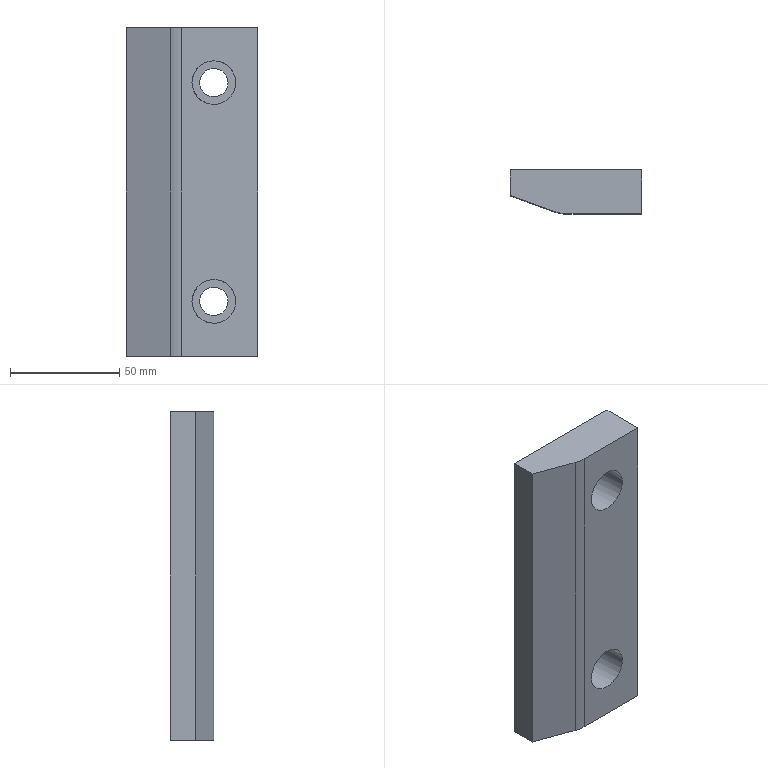Part | NX | features MAIN_BODY 2 | 1 solid | 14 faces | box 60 x 20 x 150 mm | volume 155051 mm3 | plane 9 | cylinder 5 | commonest cylinder face diameters 13 x2 20 x2 30 x1
STEP:
#1=CARTESIAN_POINT('',(-46.,-365.,-205.));
#2=VERTEX_POINT('',#1);
#3=CARTESIAN_POINT('',(14.,-365.,-205.));
#4=VERTEX_POINT('',#3);
#5=CARTESIAN_POINT('',(-71.,-365.,-205.));
#6=DIRECTION('',(1.,0.,0.));
#7=VECTOR('',#6,1000.);
#8=LINE('',#5,#7);
#9=EDGE_CURVE('',#2,#4,#8,.T.);
#10=ORIENTED_EDGE('',*,*,#9,.F.);
#11=CARTESIAN_POINT('',(-46.,-365.,-55.));
#12=VERTEX_POINT('',#11);
#13=CARTESIAN_POINT('',(-46.,-365.,-130.));
#14=DIRECTION('',(0.,0.,-1.));
#15=VECTOR('',#14,1000.);
#16=LINE('',#13,#15);
#17=EDGE_CURVE('',#12,#2,#16,.T.);
#18=ORIENTED_EDGE('',*,*,#17,.F.);
#19=CARTESIAN_POINT('',(14.,-365.,-55.));
#20=VERTEX_POINT('',#19);
#21=CARTESIAN_POINT('',(-71.,-365.,-55.));
#22=DIRECTION('',(-1.,0.,0.));
#23=VECTOR('',#22,1000.);
#24=LINE('',#21,#23);
#25=EDGE_CURVE('',#20,#12,#24,.T.);
#26=ORIENTED_EDGE('',*,*,#25,.F.);
#27=CARTESIAN_POINT('',(14.,-365.,-130.));
#28=DIRECTION('',(0.,0.,1.));
#29=VECTOR('',#28,1000.);
#30=LINE('',#27,#29);
#31=EDGE_CURVE('',#4,#20,#30,.T.);
#32=ORIENTED_EDGE('',*,*,#31,.F.);
#33=EDGE_LOOP('',(#10,#18,#26,#32));
#34=FACE_BOUND('',#33,.T.);
#35=CARTESIAN_POINT('',(-12.5,-365.,-180.));
#36=VERTEX_POINT('',#35);
#37=CARTESIAN_POINT('',(-6.,-365.,-180.));
#38=DIRECTION('',(0.,1.,0.));
#39=DIRECTION('',(-1.,0.,0.));
#40=AXIS2_PLACEMENT_3D('',#37,#38,#39);
#41=CIRCLE('',#40,6.5);
#42=EDGE_CURVE('',#36,#36,#41,.T.);
#43=ORIENTED_EDGE('',*,*,#42,.F.);
#44=EDGE_LOOP('',(#43));
#45=FACE_BOUND('',#44,.T.);
#46=CARTESIAN_POINT('',(-12.5,-365.,-80.));
#47=VERTEX_POINT('',#46);
#48=CARTESIAN_POINT('',(-6.,-365.,-80.));
#49=DIRECTION('',(0.,1.,0.));
#50=DIRECTION('',(-1.,0.,0.));
#51=AXIS2_PLACEMENT_3D('',#48,#49,#50);
#52=CIRCLE('',#51,6.5);
#53=EDGE_CURVE('',#47,#47,#52,.T.);
#54=ORIENTED_EDGE('',*,*,#53,.F.);
#55=EDGE_LOOP('',(#54));
#56=FACE_BOUND('',#55,.T.);
#57=CARTESIAN_POINT('',(-71.,-365.,-130.));
#58=DIRECTION('',(0.,1.,0.));
#59=DIRECTION('',(-1.,0.,0.));
#60=AXIS2_PLACEMENT_3D('',#57,#58,#59);
#61=PLANE('',#60);
#62=ADVANCED_FACE('',(#34,#45,#56),#61,.T.);
#63=CARTESIAN_POINT('',(14.,-385.,-205.));
#64=VERTEX_POINT('',#63);
#65=CARTESIAN_POINT('',(-20.598,-385.,-205.));
#66=VERTEX_POINT('',#65);
#67=CARTESIAN_POINT('',(-71.,-385.,-205.));
#68=DIRECTION('',(-1.,0.,0.));
#69=VECTOR('',#68,1000.);
#70=LINE('',#67,#69);
#71=EDGE_CURVE('',#64,#66,#70,.T.);
#72=ORIENTED_EDGE('',*,*,#71,.F.);
#73=CARTESIAN_POINT('',(14.,-385.,-55.));
#74=VERTEX_POINT('',#73);
#75=CARTESIAN_POINT('',(14.,-385.,-130.));
#76=DIRECTION('',(0.,0.,-1.));
#77=VECTOR('',#76,1000.);
#78=LINE('',#75,#77);
#79=EDGE_CURVE('',#74,#64,#78,.T.);
#80=ORIENTED_EDGE('',*,*,#79,.F.);
#81=CARTESIAN_POINT('',(-20.598,-385.,-55.));
#82=VERTEX_POINT('',#81);
#83=CARTESIAN_POINT('',(79.,-385.,-55.));
#84=DIRECTION('',(1.,0.,0.));
#85=VECTOR('',#84,1000.);
#86=LINE('',#83,#85);
#87=EDGE_CURVE('',#82,#74,#86,.T.);
#88=ORIENTED_EDGE('',*,*,#87,.F.);
#89=CARTESIAN_POINT('',(-20.598,-385.,-130.));
#90=DIRECTION('',(0.,0.,1.));
#91=VECTOR('',#90,1000.);
#92=LINE('',#89,#91);
#93=EDGE_CURVE('',#66,#82,#92,.T.);
#94=ORIENTED_EDGE('',*,*,#93,.F.);
#95=EDGE_LOOP('',(#72,#80,#88,#94));
#96=FACE_BOUND('',#95,.T.);
#97=CARTESIAN_POINT('',(-6.,-385.,-170.));
#98=VERTEX_POINT('',#97);
#99=CARTESIAN_POINT('',(-6.,-385.,-180.));
#100=DIRECTION('',(0.,-1.,0.));
#101=DIRECTION('',(0.,0.,1.));
#102=AXIS2_PLACEMENT_3D('',#99,#100,#101);
#103=CIRCLE('',#102,10.);
#104=EDGE_CURVE('',#98,#98,#103,.T.);
#105=ORIENTED_EDGE('',*,*,#104,.F.);
#106=EDGE_LOOP('',(#105));
#107=FACE_BOUND('',#106,.T.);
#108=CARTESIAN_POINT('',(-6.,-385.,-70.));
#109=VERTEX_POINT('',#108);
#110=CARTESIAN_POINT('',(-6.,-385.,-80.));
#111=DIRECTION('',(0.,-1.,0.));
#112=DIRECTION('',(0.,0.,1.));
#113=AXIS2_PLACEMENT_3D('',#110,#111,#112);
#114=CIRCLE('',#113,10.);
#115=EDGE_CURVE('',#109,#109,#114,.T.);
#116=ORIENTED_EDGE('',*,*,#115,.F.);
#117=EDGE_LOOP('',(#116));
#118=FACE_BOUND('',#117,.T.);
#119=CARTESIAN_POINT('',(79.,-385.,-130.));
#120=DIRECTION('',(0.,-1.,0.));
#121=DIRECTION('',(0.,0.,1.));
#122=AXIS2_PLACEMENT_3D('',#119,#120,#121);
#123=PLANE('',#122);
#124=ADVANCED_FACE('',(#96,#107,#118),#123,.T.);
#125=CARTESIAN_POINT('',(-46.,-376.717,-55.));
#126=VERTEX_POINT('',#125);
#127=CARTESIAN_POINT('',(-25.729,-384.095,-55.));
#128=VERTEX_POINT('',#127);
#129=CARTESIAN_POINT('',(-8.79,-390.261,-55.));
#130=DIRECTION('',(0.9397,-0.342,0.));
#131=VECTOR('',#130,1000.);
#132=LINE('',#129,#131);
#133=EDGE_CURVE('',#126,#128,#132,.T.);
#134=ORIENTED_EDGE('',*,*,#133,.F.);
#135=CARTESIAN_POINT('',(-46.,-376.717,-205.));
#136=VERTEX_POINT('',#135);
#137=CARTESIAN_POINT('',(-46.,-376.717,-130.));
#138=DIRECTION('',(0.,0.,1.));
#139=VECTOR('',#138,1000.);
#140=LINE('',#137,#139);
#141=EDGE_CURVE('',#136,#126,#140,.T.);
#142=ORIENTED_EDGE('',*,*,#141,.F.);
#143=CARTESIAN_POINT('',(-25.729,-384.095,-205.));
#144=VERTEX_POINT('',#143);
#145=CARTESIAN_POINT('',(-57.618,-372.489,-205.));
#146=DIRECTION('',(-0.9397,0.342,0.));
#147=VECTOR('',#146,1000.);
#148=LINE('',#145,#147);
#149=EDGE_CURVE('',#144,#136,#148,.T.);
#150=ORIENTED_EDGE('',*,*,#149,.F.);
#151=CARTESIAN_POINT('',(-25.729,-384.095,-130.));
#152=DIRECTION('',(0.,0.,1.));
#153=VECTOR('',#152,1000.);
#154=LINE('',#151,#153);
#155=EDGE_CURVE('',#128,#144,#154,.F.);
#156=ORIENTED_EDGE('',*,*,#155,.F.);
#157=EDGE_LOOP('',(#134,#142,#150,#156));
#158=FACE_BOUND('',#157,.T.);
#159=CARTESIAN_POINT('',(-8.79,-390.261,-130.));
#160=DIRECTION('',(-0.342,-0.9397,0.));
#161=DIRECTION('',(0.9397,-0.342,0.));
#162=AXIS2_PLACEMENT_3D('',#159,#160,#161);
#163=PLANE('',#162);
#164=ADVANCED_FACE('',(#158),#163,.T.);
#165=ORIENTED_EDGE('',*,*,#141,.T.);
#166=CARTESIAN_POINT('',(-46.,-395.,-55.));
#167=DIRECTION('',(0.,-1.,0.));
#168=VECTOR('',#167,1000.);
#169=LINE('',#166,#168);
#170=EDGE_CURVE('',#12,#126,#169,.T.);
#171=ORIENTED_EDGE('',*,*,#170,.F.);
#172=ORIENTED_EDGE('',*,*,#17,.T.);
#173=CARTESIAN_POINT('',(-46.,-360.359,-205.));
#174=DIRECTION('',(0.,1.,0.));
#175=VECTOR('',#174,1000.);
#176=LINE('',#173,#175);
#177=EDGE_CURVE('',#136,#2,#176,.T.);
#178=ORIENTED_EDGE('',*,*,#177,.F.);
#179=EDGE_LOOP('',(#165,#171,#172,#178));
#180=FACE_BOUND('',#179,.T.);
#181=CARTESIAN_POINT('',(-46.,-360.359,-130.));
#182=DIRECTION('',(-1.,0.,0.));
#183=DIRECTION('',(0.,0.,-1.));
#184=AXIS2_PLACEMENT_3D('',#181,#182,#183);
#185=PLANE('',#184);
#186=ADVANCED_FACE('',(#180),#185,.T.);
#187=CARTESIAN_POINT('',(14.,-395.,-205.));
#188=DIRECTION('',(0.,-1.,0.));
#189=VECTOR('',#188,1000.);
#190=LINE('',#187,#189);
#191=EDGE_CURVE('',#4,#64,#190,.T.);
#192=ORIENTED_EDGE('',*,*,#191,.F.);
#193=ORIENTED_EDGE('',*,*,#31,.T.);
#194=CARTESIAN_POINT('',(14.,-395.,-55.));
#195=DIRECTION('',(0.,-1.,0.));
#196=VECTOR('',#195,1000.);
#197=LINE('',#194,#196);
#198=EDGE_CURVE('',#20,#74,#197,.T.);
#199=ORIENTED_EDGE('',*,*,#198,.T.);
#200=ORIENTED_EDGE('',*,*,#79,.T.);
#201=EDGE_LOOP('',(#192,#193,#199,#200));
#202=FACE_BOUND('',#201,.T.);
#203=CARTESIAN_POINT('',(14.,-350.,-130.));
#204=DIRECTION('',(1.,0.,0.));
#205=DIRECTION('',(0.,0.,1.));
#206=AXIS2_PLACEMENT_3D('',#203,#204,#205);
#207=PLANE('',#206);
#208=ADVANCED_FACE('',(#202),#207,.T.);
#209=ORIENTED_EDGE('',*,*,#149,.T.);
#210=ORIENTED_EDGE('',*,*,#177,.T.);
#211=ORIENTED_EDGE('',*,*,#9,.T.);
#212=ORIENTED_EDGE('',*,*,#191,.T.);
#213=ORIENTED_EDGE('',*,*,#71,.T.);
#214=CARTESIAN_POINT('',(-20.598,-370.,-205.));
#215=DIRECTION('',(0.,0.,1.));
#216=DIRECTION('',(1.,0.,0.));
#217=AXIS2_PLACEMENT_3D('',#214,#215,#216);
#218=CIRCLE('',#217,15.);
#219=EDGE_CURVE('',#144,#66,#218,.T.);
#220=ORIENTED_EDGE('',*,*,#219,.F.);
#221=EDGE_LOOP('',(#209,#210,#211,#212,#213,#220));
#222=FACE_BOUND('',#221,.T.);
#223=CARTESIAN_POINT('',(-71.,-395.,-205.));
#224=DIRECTION('',(0.,0.,-1.));
#225=DIRECTION('',(1.,0.,0.));
#226=AXIS2_PLACEMENT_3D('',#223,#224,#225);
#227=PLANE('',#226);
#228=ADVANCED_FACE('',(#222),#227,.T.);
#229=ORIENTED_EDGE('',*,*,#42,.T.);
#230=EDGE_LOOP('',(#229));
#231=FACE_BOUND('',#230,.T.);
#232=CARTESIAN_POINT('',(-12.5,-370.,-180.));
#233=VERTEX_POINT('',#232);
#234=CARTESIAN_POINT('',(-6.,-370.,-180.));
#235=DIRECTION('',(0.,1.,0.));
#236=DIRECTION('',(-1.,0.,0.));
#237=AXIS2_PLACEMENT_3D('',#234,#235,#236);
#238=CIRCLE('',#237,6.5);
#239=EDGE_CURVE('',#233,#233,#238,.T.);
#240=ORIENTED_EDGE('',*,*,#239,.F.);
#241=EDGE_LOOP('',(#240));
#242=FACE_BOUND('',#241,.T.);
#243=CARTESIAN_POINT('',(-6.,-350.,-180.));
#244=DIRECTION('',(0.,1.,0.));
#245=DIRECTION('',(0.,0.,-1.));
#246=AXIS2_PLACEMENT_3D('',#243,#244,#245);
#247=CYLINDRICAL_SURFACE('',#246,6.5);
#248=ADVANCED_FACE('',(#231,#242),#247,.F.);
#249=ORIENTED_EDGE('',*,*,#239,.T.);
#250=EDGE_LOOP('',(#249));
#251=FACE_BOUND('',#250,.T.);
#252=CARTESIAN_POINT('',(-16.,-370.,-180.));
#253=VERTEX_POINT('',#252);
#254=CARTESIAN_POINT('',(-6.,-370.,-180.));
#255=DIRECTION('',(0.,1.,0.));
#256=DIRECTION('',(-1.,0.,0.));
#257=AXIS2_PLACEMENT_3D('',#254,#255,#256);
#258=CIRCLE('',#257,10.);
#259=EDGE_CURVE('',#253,#253,#258,.T.);
#260=ORIENTED_EDGE('',*,*,#259,.F.);
#261=EDGE_LOOP('',(#260));
#262=FACE_BOUND('',#261,.T.);
#263=CARTESIAN_POINT('',(19.,-370.,-210.));
#264=DIRECTION('',(0.,1.,0.));
#265=DIRECTION('',(0.,0.,-1.));
#266=AXIS2_PLACEMENT_3D('',#263,#264,#265);
#267=PLANE('',#266);
#268=ADVANCED_FACE('',(#251,#262),#267,.F.);
#269=ORIENTED_EDGE('',*,*,#104,.T.);
#270=EDGE_LOOP('',(#269));
#271=FACE_BOUND('',#270,.T.);
#272=ORIENTED_EDGE('',*,*,#259,.T.);
#273=EDGE_LOOP('',(#272));
#274=FACE_BOUND('',#273,.T.);
#275=CARTESIAN_POINT('',(-6.,-395.,-180.));
#276=DIRECTION('',(0.,1.,0.));
#277=DIRECTION('',(0.,0.,-1.));
#278=AXIS2_PLACEMENT_3D('',#275,#276,#277);
#279=CYLINDRICAL_SURFACE('',#278,10.);
#280=ADVANCED_FACE('',(#271,#274),#279,.F.);
#281=ORIENTED_EDGE('',*,*,#87,.T.);
#282=ORIENTED_EDGE('',*,*,#198,.F.);
#283=ORIENTED_EDGE('',*,*,#25,.T.);
#284=ORIENTED_EDGE('',*,*,#170,.T.);
#285=ORIENTED_EDGE('',*,*,#133,.T.);
#286=CARTESIAN_POINT('',(-20.598,-370.,-55.));
#287=DIRECTION('',(0.,0.,1.));
#288=DIRECTION('',(1.,0.,0.));
#289=AXIS2_PLACEMENT_3D('',#286,#287,#288);
#290=CIRCLE('',#289,15.);
#291=EDGE_CURVE('',#82,#128,#290,.F.);
#292=ORIENTED_EDGE('',*,*,#291,.F.);
#293=EDGE_LOOP('',(#281,#282,#283,#284,#285,#292));
#294=FACE_BOUND('',#293,.T.);
#295=CARTESIAN_POINT('',(-71.,-395.,-55.));
#296=DIRECTION('',(0.,0.,-1.));
#297=DIRECTION('',(1.,0.,0.));
#298=AXIS2_PLACEMENT_3D('',#295,#296,#297);
#299=PLANE('',#298);
#300=ADVANCED_FACE('',(#294),#299,.F.);
#301=ORIENTED_EDGE('',*,*,#53,.T.);
#302=EDGE_LOOP('',(#301));
#303=FACE_BOUND('',#302,.T.);
#304=CARTESIAN_POINT('',(-12.5,-370.,-80.));
#305=VERTEX_POINT('',#304);
#306=CARTESIAN_POINT('',(-6.,-370.,-80.));
#307=DIRECTION('',(0.,1.,0.));
#308=DIRECTION('',(-1.,0.,0.));
#309=AXIS2_PLACEMENT_3D('',#306,#307,#308);
#310=CIRCLE('',#309,6.5);
#311=EDGE_CURVE('',#305,#305,#310,.T.);
#312=ORIENTED_EDGE('',*,*,#311,.F.);
#313=EDGE_LOOP('',(#312));
#314=FACE_BOUND('',#313,.T.);
#315=CARTESIAN_POINT('',(-6.,-350.,-80.));
#316=DIRECTION('',(0.,1.,0.));
#317=DIRECTION('',(0.,0.,-1.));
#318=AXIS2_PLACEMENT_3D('',#315,#316,#317);
#319=CYLINDRICAL_SURFACE('',#318,6.5);
#320=ADVANCED_FACE('',(#303,#314),#319,.F.);
#321=ORIENTED_EDGE('',*,*,#311,.T.);
#322=EDGE_LOOP('',(#321));
#323=FACE_BOUND('',#322,.T.);
#324=CARTESIAN_POINT('',(-16.,-370.,-80.));
#325=VERTEX_POINT('',#324);
#326=CARTESIAN_POINT('',(-6.,-370.,-80.));
#327=DIRECTION('',(0.,1.,0.));
#328=DIRECTION('',(-1.,0.,0.));
#329=AXIS2_PLACEMENT_3D('',#326,#327,#328);
#330=CIRCLE('',#329,10.);
#331=EDGE_CURVE('',#325,#325,#330,.T.);
#332=ORIENTED_EDGE('',*,*,#331,.F.);
#333=EDGE_LOOP('',(#332));
#334=FACE_BOUND('',#333,.T.);
#335=CARTESIAN_POINT('',(19.,-370.,-135.));
#336=DIRECTION('',(0.,1.,0.));
#337=DIRECTION('',(0.,0.,-1.));
#338=AXIS2_PLACEMENT_3D('',#335,#336,#337);
#339=PLANE('',#338);
#340=ADVANCED_FACE('',(#323,#334),#339,.F.);
#341=ORIENTED_EDGE('',*,*,#115,.T.);
#342=EDGE_LOOP('',(#341));
#343=FACE_BOUND('',#342,.T.);
#344=ORIENTED_EDGE('',*,*,#331,.T.);
#345=EDGE_LOOP('',(#344));
#346=FACE_BOUND('',#345,.T.);
#347=CARTESIAN_POINT('',(-6.,-395.,-80.));
#348=DIRECTION('',(0.,1.,0.));
#349=DIRECTION('',(0.,0.,-1.));
#350=AXIS2_PLACEMENT_3D('',#347,#348,#349);
#351=CYLINDRICAL_SURFACE('',#350,10.);
#352=ADVANCED_FACE('',(#343,#346),#351,.F.);
#353=ORIENTED_EDGE('',*,*,#219,.T.);
#354=ORIENTED_EDGE('',*,*,#93,.T.);
#355=ORIENTED_EDGE('',*,*,#291,.T.);
#356=ORIENTED_EDGE('',*,*,#155,.T.);
#357=EDGE_LOOP('',(#353,#354,#355,#356));
#358=FACE_BOUND('',#357,.T.);
#359=CARTESIAN_POINT('',(-20.598,-370.,-130.));
#360=DIRECTION('',(0.,0.,1.));
#361=DIRECTION('',(-1.,0.,0.));
#362=AXIS2_PLACEMENT_3D('',#359,#360,#361);
#363=CYLINDRICAL_SURFACE('',#362,15.);
#364=ADVANCED_FACE('',(#358),#363,.T.);
#365=CLOSED_SHELL('',(#62,#124,#164,#186,#208,#228,#248,#268,#280,#300,#320,#340,#352,#364));
#366=MANIFOLD_SOLID_BREP('',#365);
#367=(LENGTH_UNIT()NAMED_UNIT(*)SI_UNIT(.MILLI.,.METRE.));
#368=UNCERTAINTY_MEASURE_WITH_UNIT(LENGTH_MEASURE(0.00001),#367,'','');
#369=(NAMED_UNIT(*)PLANE_ANGLE_UNIT()SI_UNIT($,.RADIAN.));
#370=(NAMED_UNIT(*)SI_UNIT($,.STERADIAN.)SOLID_ANGLE_UNIT());
#371=(GEOMETRIC_REPRESENTATION_CONTEXT(3)GLOBAL_UNCERTAINTY_ASSIGNED_CONTEXT((#368))GLOBAL_UNIT_ASSIGNED_CONTEXT((#367,#369,#370))REPRESENTATION_CONTEXT('',''));
#372=ADVANCED_BREP_SHAPE_REPRESENTATION('',(#366),#371);